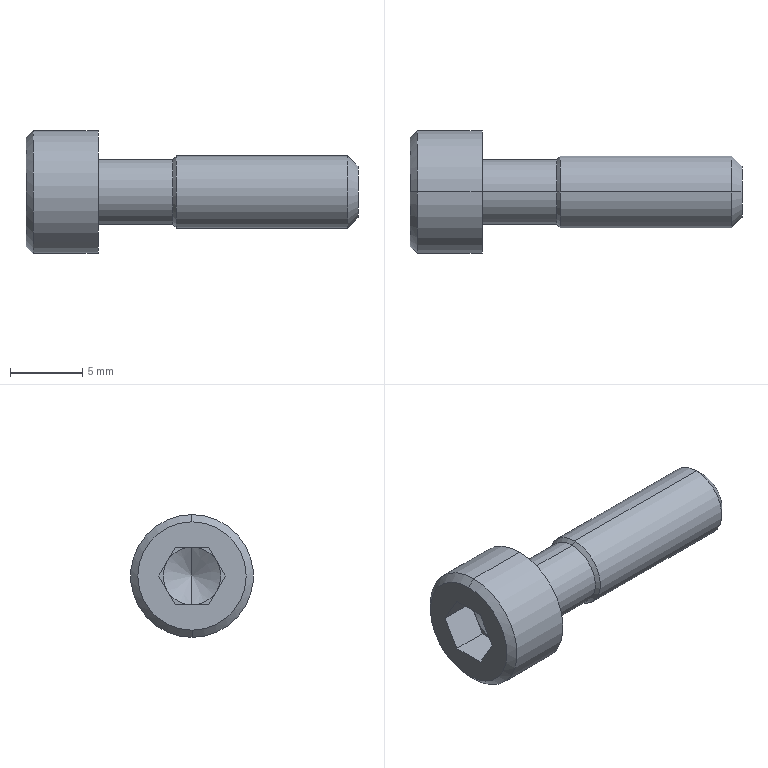Part | STEP file | 0245_312_SCB5-18_ | 1 solid | 29 faces | box 23 x 8.5 x 8.5 mm | volume 571.604 mm3 | plane 15 | cone 8 | cylinder 6 | commonest cylinder face diameters 4.509 x2 5 x2 8.5 x2